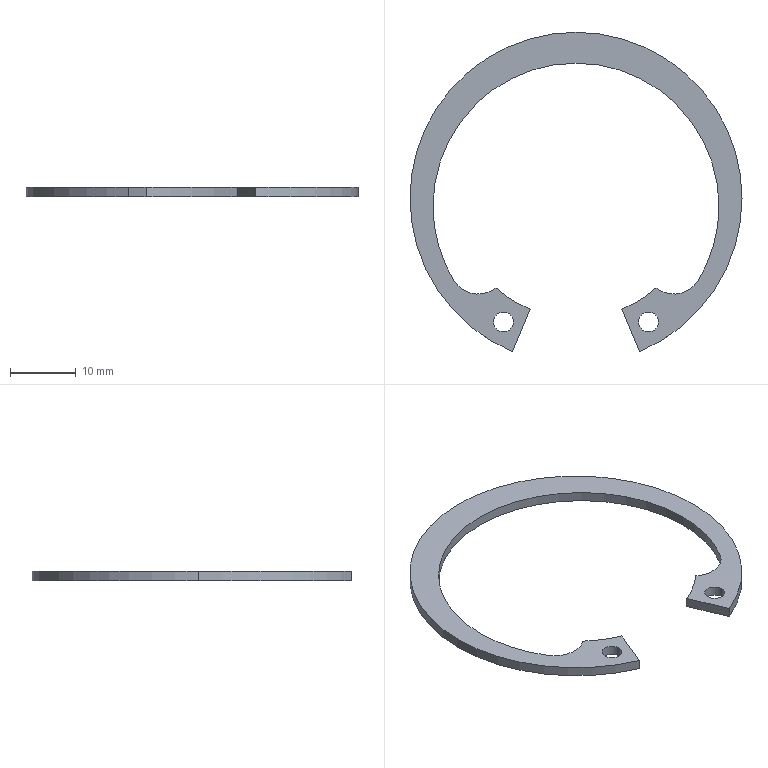Part | STEP file | circlips for hole--type b gb_GB_CONNECTING_PIECE_RINGS_CHB 47 | 1 solid | 18 faces | box 50.5 x 48.578 x 1.5 mm | volume 798.879 mm3 | cylinder 14 | plane 4 | commonest cylinder face diameters 3 x4 43.5 x3 50.5 x3 8.8 x2 36.54 x2
STEP:
#1=CARTESIAN_POINT('',(9.535,-18.801,-1.5));
#2=VERTEX_POINT('',#1);
#3=CARTESIAN_POINT('',(12.535,-18.801,-1.5));
#4=VERTEX_POINT('',#3);
#5=CARTESIAN_POINT('',(11.035,-18.801,-1.5));
#6=DIRECTION('',(0.,0.,1.));
#7=DIRECTION('',(-1.,0.,0.));
#8=AXIS2_PLACEMENT_3D('',#5,#6,#7);
#9=CIRCLE('',#8,1.5);
#10=EDGE_CURVE('',#2,#4,#9,.T.);
#11=ORIENTED_EDGE('',*,*,#10,.F.);
#12=CARTESIAN_POINT('',(9.535,-18.801,0.));
#13=VERTEX_POINT('',#12);
#14=CARTESIAN_POINT('',(9.535,-18.801,-1.5));
#15=DIRECTION('',(0.,0.,1.));
#16=VECTOR('',#15,1000.);
#17=LINE('',#14,#16);
#18=EDGE_CURVE('',#2,#13,#17,.T.);
#19=ORIENTED_EDGE('',*,*,#18,.T.);
#20=CARTESIAN_POINT('',(12.535,-18.801,0.));
#21=VERTEX_POINT('',#20);
#22=CARTESIAN_POINT('',(11.035,-18.801,0.));
#23=DIRECTION('',(0.,0.,1.));
#24=DIRECTION('',(-1.,0.,0.));
#25=AXIS2_PLACEMENT_3D('',#22,#23,#24);
#26=CIRCLE('',#25,1.5);
#27=EDGE_CURVE('',#13,#21,#26,.T.);
#28=ORIENTED_EDGE('',*,*,#27,.T.);
#29=CARTESIAN_POINT('',(12.535,-18.801,-1.5));
#30=DIRECTION('',(0.,0.,1.));
#31=VECTOR('',#30,1000.);
#32=LINE('',#29,#31);
#33=EDGE_CURVE('',#4,#21,#32,.T.);
#34=ORIENTED_EDGE('',*,*,#33,.F.);
#35=EDGE_LOOP('',(#11,#19,#28,#34));
#36=FACE_OUTER_BOUND('',#35,.T.);
#37=CARTESIAN_POINT('',(11.035,-18.801,-1.5));
#38=DIRECTION('',(0.,0.,1.));
#39=DIRECTION('',(1.,0.,0.));
#40=AXIS2_PLACEMENT_3D('',#37,#38,#39);
#41=CYLINDRICAL_SURFACE('',#40,1.5);
#42=ADVANCED_FACE('',(#36),#41,.F.);
#43=CARTESIAN_POINT('',(-12.535,-18.801,-1.5));
#44=VERTEX_POINT('',#43);
#45=CARTESIAN_POINT('',(-9.535,-18.801,-1.5));
#46=VERTEX_POINT('',#45);
#47=CARTESIAN_POINT('',(-11.035,-18.801,-1.5));
#48=DIRECTION('',(0.,0.,1.));
#49=DIRECTION('',(1.,0.,0.));
#50=AXIS2_PLACEMENT_3D('',#47,#48,#49);
#51=CIRCLE('',#50,1.5);
#52=EDGE_CURVE('',#44,#46,#51,.T.);
#53=ORIENTED_EDGE('',*,*,#52,.F.);
#54=CARTESIAN_POINT('',(-12.535,-18.801,0.));
#55=VERTEX_POINT('',#54);
#56=CARTESIAN_POINT('',(-12.535,-18.801,-1.5));
#57=DIRECTION('',(0.,0.,1.));
#58=VECTOR('',#57,1000.);
#59=LINE('',#56,#58);
#60=EDGE_CURVE('',#44,#55,#59,.T.);
#61=ORIENTED_EDGE('',*,*,#60,.T.);
#62=CARTESIAN_POINT('',(-9.535,-18.801,0.));
#63=VERTEX_POINT('',#62);
#64=CARTESIAN_POINT('',(-11.035,-18.801,0.));
#65=DIRECTION('',(0.,0.,1.));
#66=DIRECTION('',(1.,0.,0.));
#67=AXIS2_PLACEMENT_3D('',#64,#65,#66);
#68=CIRCLE('',#67,1.5);
#69=EDGE_CURVE('',#55,#63,#68,.T.);
#70=ORIENTED_EDGE('',*,*,#69,.T.);
#71=CARTESIAN_POINT('',(-9.535,-18.801,-1.5));
#72=DIRECTION('',(0.,0.,1.));
#73=VECTOR('',#72,1000.);
#74=LINE('',#71,#73);
#75=EDGE_CURVE('',#46,#63,#74,.T.);
#76=ORIENTED_EDGE('',*,*,#75,.F.);
#77=EDGE_LOOP('',(#53,#61,#70,#76));
#78=FACE_OUTER_BOUND('',#77,.T.);
#79=CARTESIAN_POINT('',(-11.035,-18.801,-1.5));
#80=DIRECTION('',(0.,0.,1.));
#81=DIRECTION('',(1.,0.,0.));
#82=AXIS2_PLACEMENT_3D('',#79,#80,#81);
#83=CYLINDRICAL_SURFACE('',#82,1.5);
#84=ADVANCED_FACE('',(#78),#83,.F.);
#85=CARTESIAN_POINT('',(-18.615,-12.45,-1.5));
#86=VERTEX_POINT('',#85);
#87=CARTESIAN_POINT('',(-21.75,-1.2,-1.5));
#88=VERTEX_POINT('',#87);
#89=CARTESIAN_POINT('',(0.,-1.2,-1.5));
#90=DIRECTION('',(0.,0.,-1.));
#91=DIRECTION('',(1.,0.,0.));
#92=AXIS2_PLACEMENT_3D('',#89,#90,#91);
#93=CIRCLE('',#92,21.75);
#94=EDGE_CURVE('',#86,#88,#93,.T.);
#95=ORIENTED_EDGE('',*,*,#94,.T.);
#96=CARTESIAN_POINT('',(-21.75,-1.2,0.));
#97=VERTEX_POINT('',#96);
#98=CARTESIAN_POINT('',(-21.75,-1.2,-1.5));
#99=DIRECTION('',(0.,0.,1.));
#100=VECTOR('',#99,1000.);
#101=LINE('',#98,#100);
#102=EDGE_CURVE('',#88,#97,#101,.T.);
#103=ORIENTED_EDGE('',*,*,#102,.T.);
#104=CARTESIAN_POINT('',(-18.615,-12.45,0.));
#105=VERTEX_POINT('',#104);
#106=CARTESIAN_POINT('',(0.,-1.2,0.));
#107=DIRECTION('',(0.,0.,-1.));
#108=DIRECTION('',(1.,0.,0.));
#109=AXIS2_PLACEMENT_3D('',#106,#107,#108);
#110=CIRCLE('',#109,21.75);
#111=EDGE_CURVE('',#105,#97,#110,.T.);
#112=ORIENTED_EDGE('',*,*,#111,.F.);
#113=CARTESIAN_POINT('',(-18.615,-12.45,-1.5));
#114=DIRECTION('',(0.,0.,1.));
#115=VECTOR('',#114,1000.);
#116=LINE('',#113,#115);
#117=EDGE_CURVE('',#86,#105,#116,.T.);
#118=ORIENTED_EDGE('',*,*,#117,.F.);
#119=EDGE_LOOP('',(#95,#103,#112,#118));
#120=FACE_OUTER_BOUND('',#119,.T.);
#121=CARTESIAN_POINT('',(0.,-1.2,-1.5));
#122=DIRECTION('',(0.,0.,1.));
#123=DIRECTION('',(1.,0.,0.));
#124=AXIS2_PLACEMENT_3D('',#121,#122,#123);
#125=CYLINDRICAL_SURFACE('',#124,21.75);
#126=ADVANCED_FACE('',(#120),#125,.F.);
#127=ORIENTED_EDGE('',*,*,#102,.F.);
#128=CARTESIAN_POINT('',(21.75,-1.2,-1.5));
#129=VERTEX_POINT('',#128);
#130=CARTESIAN_POINT('',(0.,-1.2,-1.5));
#131=DIRECTION('',(0.,0.,-1.));
#132=DIRECTION('',(1.,0.,0.));
#133=AXIS2_PLACEMENT_3D('',#130,#131,#132);
#134=CIRCLE('',#133,21.75);
#135=EDGE_CURVE('',#88,#129,#134,.T.);
#136=ORIENTED_EDGE('',*,*,#135,.T.);
#137=CARTESIAN_POINT('',(21.75,-1.2,0.));
#138=VERTEX_POINT('',#137);
#139=CARTESIAN_POINT('',(21.75,-1.2,-1.5));
#140=DIRECTION('',(0.,0.,1.));
#141=VECTOR('',#140,1000.);
#142=LINE('',#139,#141);
#143=EDGE_CURVE('',#129,#138,#142,.T.);
#144=ORIENTED_EDGE('',*,*,#143,.T.);
#145=CARTESIAN_POINT('',(0.,-1.2,0.));
#146=DIRECTION('',(0.,0.,-1.));
#147=DIRECTION('',(1.,0.,0.));
#148=AXIS2_PLACEMENT_3D('',#145,#146,#147);
#149=CIRCLE('',#148,21.75);
#150=EDGE_CURVE('',#97,#138,#149,.T.);
#151=ORIENTED_EDGE('',*,*,#150,.F.);
#152=EDGE_LOOP('',(#127,#136,#144,#151));
#153=FACE_OUTER_BOUND('',#152,.T.);
#154=CARTESIAN_POINT('',(0.,-1.2,-1.5));
#155=DIRECTION('',(0.,0.,1.));
#156=DIRECTION('',(1.,0.,0.));
#157=AXIS2_PLACEMENT_3D('',#154,#155,#156);
#158=CYLINDRICAL_SURFACE('',#157,21.75);
#159=ADVANCED_FACE('',(#153),#158,.F.);
#160=CARTESIAN_POINT('',(25.25,0.,-1.5));
#161=VERTEX_POINT('',#160);
#162=CARTESIAN_POINT('',(-25.25,0.,-1.5));
#163=VERTEX_POINT('',#162);
#164=CARTESIAN_POINT('',(0.,0.,-1.5));
#165=DIRECTION('',(0.,0.,1.));
#166=DIRECTION('',(1.,0.,0.));
#167=AXIS2_PLACEMENT_3D('',#164,#165,#166);
#168=CIRCLE('',#167,25.25);
#169=EDGE_CURVE('',#161,#163,#168,.T.);
#170=ORIENTED_EDGE('',*,*,#169,.T.);
#171=CARTESIAN_POINT('',(-25.25,0.,0.));
#172=VERTEX_POINT('',#171);
#173=CARTESIAN_POINT('',(-25.25,0.,-1.5));
#174=DIRECTION('',(0.,0.,1.));
#175=VECTOR('',#174,1000.);
#176=LINE('',#173,#175);
#177=EDGE_CURVE('',#163,#172,#176,.T.);
#178=ORIENTED_EDGE('',*,*,#177,.T.);
#179=CARTESIAN_POINT('',(25.25,0.,0.));
#180=VERTEX_POINT('',#179);
#181=CARTESIAN_POINT('',(0.,0.,0.));
#182=DIRECTION('',(0.,0.,1.));
#183=DIRECTION('',(1.,0.,0.));
#184=AXIS2_PLACEMENT_3D('',#181,#182,#183);
#185=CIRCLE('',#184,25.25);
#186=EDGE_CURVE('',#180,#172,#185,.T.);
#187=ORIENTED_EDGE('',*,*,#186,.F.);
#188=CARTESIAN_POINT('',(25.25,0.,-1.5));
#189=DIRECTION('',(0.,0.,1.));
#190=VECTOR('',#189,1000.);
#191=LINE('',#188,#190);
#192=EDGE_CURVE('',#161,#180,#191,.T.);
#193=ORIENTED_EDGE('',*,*,#192,.F.);
#194=EDGE_LOOP('',(#170,#178,#187,#193));
#195=FACE_OUTER_BOUND('',#194,.T.);
#196=CARTESIAN_POINT('',(0.,0.,-1.5));
#197=DIRECTION('',(0.,0.,1.));
#198=DIRECTION('',(1.,0.,0.));
#199=AXIS2_PLACEMENT_3D('',#196,#197,#198);
#200=CYLINDRICAL_SURFACE('',#199,25.25);
#201=ADVANCED_FACE('',(#195),#200,.T.);
#202=CARTESIAN_POINT('',(9.663,-23.328,-1.5));
#203=VERTEX_POINT('',#202);
#204=CARTESIAN_POINT('',(0.,0.,-1.5));
#205=DIRECTION('',(0.,0.,1.));
#206=DIRECTION('',(1.,0.,0.));
#207=AXIS2_PLACEMENT_3D('',#204,#205,#206);
#208=CIRCLE('',#207,25.25);
#209=EDGE_CURVE('',#203,#161,#208,.T.);
#210=ORIENTED_EDGE('',*,*,#209,.T.);
#211=ORIENTED_EDGE('',*,*,#192,.T.);
#212=CARTESIAN_POINT('',(9.663,-23.328,0.));
#213=VERTEX_POINT('',#212);
#214=CARTESIAN_POINT('',(0.,0.,0.));
#215=DIRECTION('',(0.,0.,1.));
#216=DIRECTION('',(1.,0.,0.));
#217=AXIS2_PLACEMENT_3D('',#214,#215,#216);
#218=CIRCLE('',#217,25.25);
#219=EDGE_CURVE('',#213,#180,#218,.T.);
#220=ORIENTED_EDGE('',*,*,#219,.F.);
#221=CARTESIAN_POINT('',(9.663,-23.328,-1.5));
#222=DIRECTION('',(0.,0.,1.));
#223=VECTOR('',#222,1000.);
#224=LINE('',#221,#223);
#225=EDGE_CURVE('',#203,#213,#224,.T.);
#226=ORIENTED_EDGE('',*,*,#225,.F.);
#227=EDGE_LOOP('',(#210,#211,#220,#226));
#228=FACE_OUTER_BOUND('',#227,.T.);
#229=CARTESIAN_POINT('',(0.,0.,-1.5));
#230=DIRECTION('',(0.,0.,1.));
#231=DIRECTION('',(1.,0.,0.));
#232=AXIS2_PLACEMENT_3D('',#229,#230,#231);
#233=CYLINDRICAL_SURFACE('',#232,25.25);
#234=ADVANCED_FACE('',(#228),#233,.T.);
#235=ORIENTED_EDGE('',*,*,#177,.F.);
#236=CARTESIAN_POINT('',(-9.663,-23.328,-1.5));
#237=VERTEX_POINT('',#236);
#238=CARTESIAN_POINT('',(0.,0.,-1.5));
#239=DIRECTION('',(0.,0.,1.));
#240=DIRECTION('',(1.,0.,0.));
#241=AXIS2_PLACEMENT_3D('',#238,#239,#240);
#242=CIRCLE('',#241,25.25);
#243=EDGE_CURVE('',#163,#237,#242,.T.);
#244=ORIENTED_EDGE('',*,*,#243,.T.);
#245=CARTESIAN_POINT('',(-9.663,-23.328,0.));
#246=VERTEX_POINT('',#245);
#247=CARTESIAN_POINT('',(-9.663,-23.328,-1.5));
#248=DIRECTION('',(0.,0.,1.));
#249=VECTOR('',#248,1000.);
#250=LINE('',#247,#249);
#251=EDGE_CURVE('',#237,#246,#250,.T.);
#252=ORIENTED_EDGE('',*,*,#251,.T.);
#253=CARTESIAN_POINT('',(0.,0.,0.));
#254=DIRECTION('',(0.,0.,1.));
#255=DIRECTION('',(1.,0.,0.));
#256=AXIS2_PLACEMENT_3D('',#253,#254,#255);
#257=CIRCLE('',#256,25.25);
#258=EDGE_CURVE('',#172,#246,#257,.T.);
#259=ORIENTED_EDGE('',*,*,#258,.F.);
#260=EDGE_LOOP('',(#235,#244,#252,#259));
#261=FACE_OUTER_BOUND('',#260,.T.);
#262=CARTESIAN_POINT('',(0.,0.,-1.5));
#263=DIRECTION('',(0.,0.,1.));
#264=DIRECTION('',(1.,0.,0.));
#265=AXIS2_PLACEMENT_3D('',#262,#263,#264);
#266=CYLINDRICAL_SURFACE('',#265,25.25);
#267=ADVANCED_FACE('',(#261),#266,.T.);
#268=CARTESIAN_POINT('',(6.992,-16.879,0.));
#269=VERTEX_POINT('',#268);
#270=CARTESIAN_POINT('',(6.992,-16.879,0.));
#271=DIRECTION('',(0.3827,-0.9239,0.));
#272=VECTOR('',#271,1000.);
#273=LINE('',#270,#272);
#274=EDGE_CURVE('',#269,#213,#273,.T.);
#275=ORIENTED_EDGE('',*,*,#274,.F.);
#276=CARTESIAN_POINT('',(6.992,-16.879,-1.5));
#277=VERTEX_POINT('',#276);
#278=CARTESIAN_POINT('',(6.992,-16.879,-1.5));
#279=DIRECTION('',(0.,0.,1.));
#280=VECTOR('',#279,1000.);
#281=LINE('',#278,#280);
#282=EDGE_CURVE('',#277,#269,#281,.T.);
#283=ORIENTED_EDGE('',*,*,#282,.F.);
#284=CARTESIAN_POINT('',(6.992,-16.879,-1.5));
#285=DIRECTION('',(0.3827,-0.9239,0.));
#286=VECTOR('',#285,1000.);
#287=LINE('',#284,#286);
#288=EDGE_CURVE('',#277,#203,#287,.T.);
#289=ORIENTED_EDGE('',*,*,#288,.T.);
#290=ORIENTED_EDGE('',*,*,#225,.T.);
#291=EDGE_LOOP('',(#275,#283,#289,#290));
#292=FACE_OUTER_BOUND('',#291,.T.);
#293=CARTESIAN_POINT('',(6.992,-16.879,-1.5));
#294=DIRECTION('',(-0.9239,-0.3827,0.));
#295=DIRECTION('',(0.3827,-0.9239,0.));
#296=AXIS2_PLACEMENT_3D('',#293,#294,#295);
#297=PLANE('',#296);
#298=ADVANCED_FACE('',(#292),#297,.T.);
#299=CARTESIAN_POINT('',(12.147,-13.647,0.));
#300=VERTEX_POINT('',#299);
#301=CARTESIAN_POINT('',(0.,0.,0.));
#302=DIRECTION('',(0.,0.,-1.));
#303=DIRECTION('',(-1.,0.,0.));
#304=AXIS2_PLACEMENT_3D('',#301,#302,#303);
#305=CIRCLE('',#304,18.27);
#306=EDGE_CURVE('',#300,#269,#305,.T.);
#307=ORIENTED_EDGE('',*,*,#306,.F.);
#308=CARTESIAN_POINT('',(12.147,-13.647,-1.5));
#309=VERTEX_POINT('',#308);
#310=CARTESIAN_POINT('',(12.147,-13.647,-1.5));
#311=DIRECTION('',(0.,0.,1.));
#312=VECTOR('',#311,1000.);
#313=LINE('',#310,#312);
#314=EDGE_CURVE('',#309,#300,#313,.T.);
#315=ORIENTED_EDGE('',*,*,#314,.F.);
#316=CARTESIAN_POINT('',(0.,0.,-1.5));
#317=DIRECTION('',(0.,0.,-1.));
#318=DIRECTION('',(-1.,0.,0.));
#319=AXIS2_PLACEMENT_3D('',#316,#317,#318);
#320=CIRCLE('',#319,18.27);
#321=EDGE_CURVE('',#309,#277,#320,.T.);
#322=ORIENTED_EDGE('',*,*,#321,.T.);
#323=ORIENTED_EDGE('',*,*,#282,.T.);
#324=EDGE_LOOP('',(#307,#315,#322,#323));
#325=FACE_OUTER_BOUND('',#324,.T.);
#326=CARTESIAN_POINT('',(0.,0.,-1.5));
#327=DIRECTION('',(0.,0.,1.));
#328=DIRECTION('',(1.,0.,0.));
#329=AXIS2_PLACEMENT_3D('',#326,#327,#328);
#330=CYLINDRICAL_SURFACE('',#329,18.27);
#331=ADVANCED_FACE('',(#325),#330,.F.);
#332=CARTESIAN_POINT('',(18.615,-12.45,0.));
#333=VERTEX_POINT('',#332);
#334=CARTESIAN_POINT('',(14.849,-10.174,0.));
#335=DIRECTION('',(0.,0.,-1.));
#336=DIRECTION('',(-1.,0.,0.));
#337=AXIS2_PLACEMENT_3D('',#334,#335,#336);
#338=CIRCLE('',#337,4.4);
#339=EDGE_CURVE('',#333,#300,#338,.T.);
#340=ORIENTED_EDGE('',*,*,#339,.F.);
#341=CARTESIAN_POINT('',(18.615,-12.45,-1.5));
#342=VERTEX_POINT('',#341);
#343=CARTESIAN_POINT('',(18.615,-12.45,-1.5));
#344=DIRECTION('',(0.,0.,1.));
#345=VECTOR('',#344,1000.);
#346=LINE('',#343,#345);
#347=EDGE_CURVE('',#342,#333,#346,.T.);
#348=ORIENTED_EDGE('',*,*,#347,.F.);
#349=CARTESIAN_POINT('',(14.849,-10.174,-1.5));
#350=DIRECTION('',(0.,0.,-1.));
#351=DIRECTION('',(-1.,0.,0.));
#352=AXIS2_PLACEMENT_3D('',#349,#350,#351);
#353=CIRCLE('',#352,4.4);
#354=EDGE_CURVE('',#342,#309,#353,.T.);
#355=ORIENTED_EDGE('',*,*,#354,.T.);
#356=ORIENTED_EDGE('',*,*,#314,.T.);
#357=EDGE_LOOP('',(#340,#348,#355,#356));
#358=FACE_OUTER_BOUND('',#357,.T.);
#359=CARTESIAN_POINT('',(14.849,-10.174,-1.5));
#360=DIRECTION('',(0.,0.,1.));
#361=DIRECTION('',(1.,0.,0.));
#362=AXIS2_PLACEMENT_3D('',#359,#360,#361);
#363=CYLINDRICAL_SURFACE('',#362,4.4);
#364=ADVANCED_FACE('',(#358),#363,.F.);
#365=ORIENTED_EDGE('',*,*,#143,.F.);
#366=CARTESIAN_POINT('',(0.,-1.2,-1.5));
#367=DIRECTION('',(0.,0.,-1.));
#368=DIRECTION('',(1.,0.,0.));
#369=AXIS2_PLACEMENT_3D('',#366,#367,#368);
#370=CIRCLE('',#369,21.75);
#371=EDGE_CURVE('',#129,#342,#370,.T.);
#372=ORIENTED_EDGE('',*,*,#371,.T.);
#373=ORIENTED_EDGE('',*,*,#347,.T.);
#374=CARTESIAN_POINT('',(0.,-1.2,0.));
#375=DIRECTION('',(0.,0.,-1.));
#376=DIRECTION('',(1.,0.,0.));
#377=AXIS2_PLACEMENT_3D('',#374,#375,#376);
#378=CIRCLE('',#377,21.75);
#379=EDGE_CURVE('',#138,#333,#378,.T.);
#380=ORIENTED_EDGE('',*,*,#379,.F.);
#381=EDGE_LOOP('',(#365,#372,#373,#380));
#382=FACE_OUTER_BOUND('',#381,.T.);
#383=CARTESIAN_POINT('',(0.,-1.2,-1.5));
#384=DIRECTION('',(0.,0.,1.));
#385=DIRECTION('',(1.,0.,0.));
#386=AXIS2_PLACEMENT_3D('',#383,#384,#385);
#387=CYLINDRICAL_SURFACE('',#386,21.75);
#388=ADVANCED_FACE('',(#382),#387,.F.);
#389=CARTESIAN_POINT('',(-12.147,-13.647,0.));
#390=VERTEX_POINT('',#389);
#391=CARTESIAN_POINT('',(-14.849,-10.174,0.));
#392=DIRECTION('',(0.,0.,-1.));
#393=DIRECTION('',(1.,0.,0.));
#394=AXIS2_PLACEMENT_3D('',#391,#392,#393);
#395=CIRCLE('',#394,4.4);
#396=EDGE_CURVE('',#390,#105,#395,.T.);
#397=ORIENTED_EDGE('',*,*,#396,.F.);
#398=CARTESIAN_POINT('',(-12.147,-13.647,-1.5));
#399=VERTEX_POINT('',#398);
#400=CARTESIAN_POINT('',(-12.147,-13.647,-1.5));
#401=DIRECTION('',(0.,0.,1.));
#402=VECTOR('',#401,1000.);
#403=LINE('',#400,#402);
#404=EDGE_CURVE('',#399,#390,#403,.T.);
#405=ORIENTED_EDGE('',*,*,#404,.F.);
#406=CARTESIAN_POINT('',(-14.849,-10.174,-1.5));
#407=DIRECTION('',(0.,0.,-1.));
#408=DIRECTION('',(1.,0.,0.));
#409=AXIS2_PLACEMENT_3D('',#406,#407,#408);
#410=CIRCLE('',#409,4.4);
#411=EDGE_CURVE('',#399,#86,#410,.T.);
#412=ORIENTED_EDGE('',*,*,#411,.T.);
#413=ORIENTED_EDGE('',*,*,#117,.T.);
#414=EDGE_LOOP('',(#397,#405,#412,#413));
#415=FACE_OUTER_BOUND('',#414,.T.);
#416=CARTESIAN_POINT('',(-14.849,-10.174,-1.5));
#417=DIRECTION('',(0.,0.,1.));
#418=DIRECTION('',(1.,0.,0.));
#419=AXIS2_PLACEMENT_3D('',#416,#417,#418);
#420=CYLINDRICAL_SURFACE('',#419,4.4);
#421=ADVANCED_FACE('',(#415),#420,.F.);
#422=CARTESIAN_POINT('',(-6.992,-16.879,0.));
#423=VERTEX_POINT('',#422);
#424=CARTESIAN_POINT('',(0.,0.,0.));
#425=DIRECTION('',(0.,0.,-1.));
#426=DIRECTION('',(1.,0.,0.));
#427=AXIS2_PLACEMENT_3D('',#424,#425,#426);
#428=CIRCLE('',#427,18.27);
#429=EDGE_CURVE('',#423,#390,#428,.T.);
#430=ORIENTED_EDGE('',*,*,#429,.F.);
#431=CARTESIAN_POINT('',(-6.992,-16.879,-1.5));
#432=VERTEX_POINT('',#431);
#433=CARTESIAN_POINT('',(-6.992,-16.879,-1.5));
#434=DIRECTION('',(0.,0.,1.));
#435=VECTOR('',#434,1000.);
#436=LINE('',#433,#435);
#437=EDGE_CURVE('',#432,#423,#436,.T.);
#438=ORIENTED_EDGE('',*,*,#437,.F.);
#439=CARTESIAN_POINT('',(0.,0.,-1.5));
#440=DIRECTION('',(0.,0.,-1.));
#441=DIRECTION('',(1.,0.,0.));
#442=AXIS2_PLACEMENT_3D('',#439,#440,#441);
#443=CIRCLE('',#442,18.27);
#444=EDGE_CURVE('',#432,#399,#443,.T.);
#445=ORIENTED_EDGE('',*,*,#444,.T.);
#446=ORIENTED_EDGE('',*,*,#404,.T.);
#447=EDGE_LOOP('',(#430,#438,#445,#446));
#448=FACE_OUTER_BOUND('',#447,.T.);
#449=CARTESIAN_POINT('',(0.,0.,-1.5));
#450=DIRECTION('',(0.,0.,1.));
#451=DIRECTION('',(1.,0.,0.));
#452=AXIS2_PLACEMENT_3D('',#449,#450,#451);
#453=CYLINDRICAL_SURFACE('',#452,18.27);
#454=ADVANCED_FACE('',(#448),#453,.F.);
#455=CARTESIAN_POINT('',(-6.992,-16.879,0.));
#456=DIRECTION('',(0.3827,0.9239,0.));
#457=VECTOR('',#456,1000.);
#458=LINE('',#455,#457);
#459=EDGE_CURVE('',#246,#423,#458,.T.);
#460=ORIENTED_EDGE('',*,*,#459,.F.);
#461=ORIENTED_EDGE('',*,*,#251,.F.);
#462=CARTESIAN_POINT('',(-6.992,-16.879,-1.5));
#463=DIRECTION('',(0.3827,0.9239,0.));
#464=VECTOR('',#463,1000.);
#465=LINE('',#462,#464);
#466=EDGE_CURVE('',#237,#432,#465,.T.);
#467=ORIENTED_EDGE('',*,*,#466,.T.);
#468=ORIENTED_EDGE('',*,*,#437,.T.);
#469=EDGE_LOOP('',(#460,#461,#467,#468));
#470=FACE_OUTER_BOUND('',#469,.T.);
#471=CARTESIAN_POINT('',(-6.992,-16.879,-1.5));
#472=DIRECTION('',(0.9239,-0.3827,0.));
#473=DIRECTION('',(0.3827,0.9239,0.));
#474=AXIS2_PLACEMENT_3D('',#471,#472,#473);
#475=PLANE('',#474);
#476=ADVANCED_FACE('',(#470),#475,.T.);
#477=CARTESIAN_POINT('',(11.035,-18.801,-1.5));
#478=DIRECTION('',(0.,0.,1.));
#479=DIRECTION('',(-1.,0.,0.));
#480=AXIS2_PLACEMENT_3D('',#477,#478,#479);
#481=CIRCLE('',#480,1.5);
#482=EDGE_CURVE('',#4,#2,#481,.T.);
#483=ORIENTED_EDGE('',*,*,#482,.T.);
#484=ORIENTED_EDGE('',*,*,#10,.T.);
#485=EDGE_LOOP('',(#483,#484));
#486=FACE_BOUND('',#485,.T.);
#487=CARTESIAN_POINT('',(-11.035,-18.801,-1.5));
#488=DIRECTION('',(0.,0.,1.));
#489=DIRECTION('',(1.,0.,0.));
#490=AXIS2_PLACEMENT_3D('',#487,#488,#489);
#491=CIRCLE('',#490,1.5);
#492=EDGE_CURVE('',#46,#44,#491,.T.);
#493=ORIENTED_EDGE('',*,*,#492,.T.);
#494=ORIENTED_EDGE('',*,*,#52,.T.);
#495=EDGE_LOOP('',(#493,#494));
#496=FACE_BOUND('',#495,.T.);
#497=ORIENTED_EDGE('',*,*,#209,.F.);
#498=ORIENTED_EDGE('',*,*,#288,.F.);
#499=ORIENTED_EDGE('',*,*,#321,.F.);
#500=ORIENTED_EDGE('',*,*,#354,.F.);
#501=ORIENTED_EDGE('',*,*,#371,.F.);
#502=ORIENTED_EDGE('',*,*,#135,.F.);
#503=ORIENTED_EDGE('',*,*,#94,.F.);
#504=ORIENTED_EDGE('',*,*,#411,.F.);
#505=ORIENTED_EDGE('',*,*,#444,.F.);
#506=ORIENTED_EDGE('',*,*,#466,.F.);
#507=ORIENTED_EDGE('',*,*,#243,.F.);
#508=ORIENTED_EDGE('',*,*,#169,.F.);
#509=EDGE_LOOP('',(#497,#498,#499,#500,#501,#502,#503,#504,#505,#506,#507,#508));
#510=FACE_OUTER_BOUND('',#509,.T.);
#511=CARTESIAN_POINT('',(0.,0.,-1.5));
#512=DIRECTION('',(0.,0.,1.));
#513=DIRECTION('',(1.,0.,0.));
#514=AXIS2_PLACEMENT_3D('',#511,#512,#513);
#515=PLANE('',#514);
#516=ADVANCED_FACE('',(#486,#496,#510),#515,.F.);
#517=CARTESIAN_POINT('',(11.035,-18.801,0.));
#518=DIRECTION('',(0.,0.,1.));
#519=DIRECTION('',(-1.,0.,0.));
#520=AXIS2_PLACEMENT_3D('',#517,#518,#519);
#521=CIRCLE('',#520,1.5);
#522=EDGE_CURVE('',#21,#13,#521,.T.);
#523=ORIENTED_EDGE('',*,*,#522,.F.);
#524=ORIENTED_EDGE('',*,*,#27,.F.);
#525=EDGE_LOOP('',(#523,#524));
#526=FACE_BOUND('',#525,.T.);
#527=CARTESIAN_POINT('',(-11.035,-18.801,0.));
#528=DIRECTION('',(0.,0.,1.));
#529=DIRECTION('',(1.,0.,0.));
#530=AXIS2_PLACEMENT_3D('',#527,#528,#529);
#531=CIRCLE('',#530,1.5);
#532=EDGE_CURVE('',#63,#55,#531,.T.);
#533=ORIENTED_EDGE('',*,*,#532,.F.);
#534=ORIENTED_EDGE('',*,*,#69,.F.);
#535=EDGE_LOOP('',(#533,#534));
#536=FACE_BOUND('',#535,.T.);
#537=ORIENTED_EDGE('',*,*,#219,.T.);
#538=ORIENTED_EDGE('',*,*,#186,.T.);
#539=ORIENTED_EDGE('',*,*,#258,.T.);
#540=ORIENTED_EDGE('',*,*,#459,.T.);
#541=ORIENTED_EDGE('',*,*,#429,.T.);
#542=ORIENTED_EDGE('',*,*,#396,.T.);
#543=ORIENTED_EDGE('',*,*,#111,.T.);
#544=ORIENTED_EDGE('',*,*,#150,.T.);
#545=ORIENTED_EDGE('',*,*,#379,.T.);
#546=ORIENTED_EDGE('',*,*,#339,.T.);
#547=ORIENTED_EDGE('',*,*,#306,.T.);
#548=ORIENTED_EDGE('',*,*,#274,.T.);
#549=EDGE_LOOP('',(#537,#538,#539,#540,#541,#542,#543,#544,#545,#546,#547,#548));
#550=FACE_OUTER_BOUND('',#549,.T.);
#551=CARTESIAN_POINT('',(0.,0.,0.));
#552=DIRECTION('',(0.,0.,1.));
#553=DIRECTION('',(1.,0.,0.));
#554=AXIS2_PLACEMENT_3D('',#551,#552,#553);
#555=PLANE('',#554);
#556=ADVANCED_FACE('',(#526,#536,#550),#555,.T.);
#557=ORIENTED_EDGE('',*,*,#60,.F.);
#558=ORIENTED_EDGE('',*,*,#492,.F.);
#559=ORIENTED_EDGE('',*,*,#75,.T.);
#560=ORIENTED_EDGE('',*,*,#532,.T.);
#561=EDGE_LOOP('',(#557,#558,#559,#560));
#562=FACE_OUTER_BOUND('',#561,.T.);
#563=CARTESIAN_POINT('',(-11.035,-18.801,-1.5));
#564=DIRECTION('',(0.,0.,1.));
#565=DIRECTION('',(1.,0.,0.));
#566=AXIS2_PLACEMENT_3D('',#563,#564,#565);
#567=CYLINDRICAL_SURFACE('',#566,1.5);
#568=ADVANCED_FACE('',(#562),#567,.F.);
#569=ORIENTED_EDGE('',*,*,#18,.F.);
#570=ORIENTED_EDGE('',*,*,#482,.F.);
#571=ORIENTED_EDGE('',*,*,#33,.T.);
#572=ORIENTED_EDGE('',*,*,#522,.T.);
#573=EDGE_LOOP('',(#569,#570,#571,#572));
#574=FACE_OUTER_BOUND('',#573,.T.);
#575=CARTESIAN_POINT('',(11.035,-18.801,-1.5));
#576=DIRECTION('',(0.,0.,1.));
#577=DIRECTION('',(1.,0.,0.));
#578=AXIS2_PLACEMENT_3D('',#575,#576,#577);
#579=CYLINDRICAL_SURFACE('',#578,1.5);
#580=ADVANCED_FACE('',(#574),#579,.F.);
#581=CLOSED_SHELL('',(#42,#84,#126,#159,#201,#234,#267,#298,#331,#364,#388,#421,#454,#476,#516,#556,#568,#580));
#582=MANIFOLD_SOLID_BREP('',#581);
#583=CARTESIAN_POINT('',(0.,0.,0.));
#584=DIRECTION('',(0.,0.,1.));
#585=DIRECTION('',(1.,0.,0.));
#586=AXIS2_PLACEMENT_3D('',#583,#584,#585);
#587=(LENGTH_UNIT()NAMED_UNIT(*)SI_UNIT(.MILLI.,.METRE.));
#588=UNCERTAINTY_MEASURE_WITH_UNIT(LENGTH_MEASURE(0.00001),#587,'','');
#589=(NAMED_UNIT(*)PLANE_ANGLE_UNIT()SI_UNIT($,.RADIAN.));
#590=(NAMED_UNIT(*)SI_UNIT($,.STERADIAN.)SOLID_ANGLE_UNIT());
#591=(GEOMETRIC_REPRESENTATION_CONTEXT(3)GLOBAL_UNCERTAINTY_ASSIGNED_CONTEXT((#588))GLOBAL_UNIT_ASSIGNED_CONTEXT((#587,#589,#590))REPRESENTATION_CONTEXT('',''));
#592=ADVANCED_BREP_SHAPE_REPRESENTATION('',(#582,#586),#591);